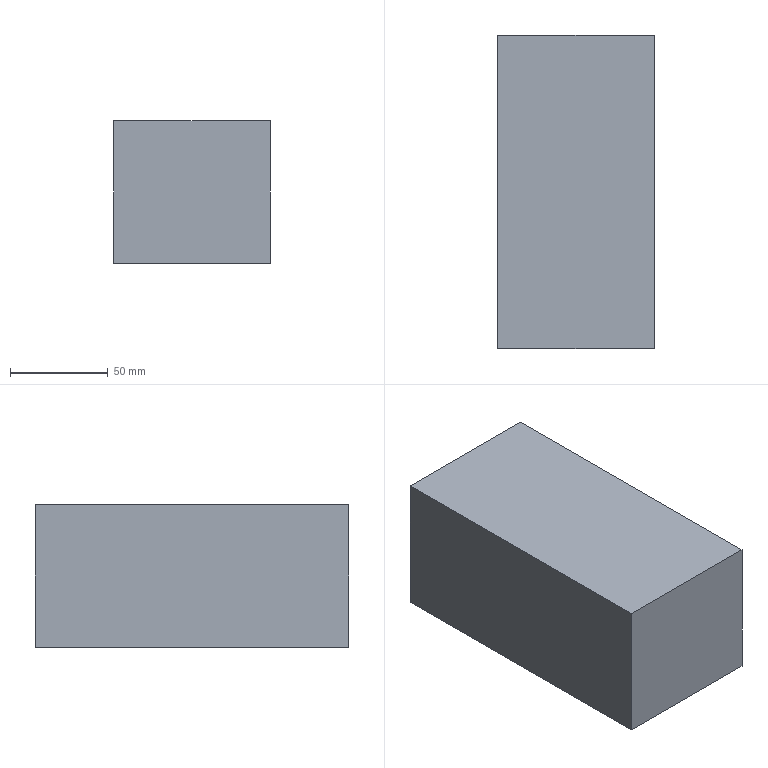Part | STEP file | 1 solid | 12 faces | box 80 x 160 x 72.8 mm | volume 929967 mm3 | plane 6 | cone 4 | cylinder 2 | commonest cylinder face diameters 6.8 x2
STEP:
#1=CARTESIAN_POINT('',(0.,0.,0.));
#2=DIRECTION('',(0.,0.,1.));
#3=DIRECTION('',(1.,0.,0.));
#4=AXIS2_PLACEMENT_3D('',#1,#2,#3);
#5=CARTESIAN_POINT('',(1936.247,362.48,-22.581));
#6=VERTEX_POINT('',#5);
#7=CARTESIAN_POINT('',(1856.247,362.48,-22.581));
#8=VERTEX_POINT('',#7);
#9=CARTESIAN_POINT('',(1956.247,362.48,-22.581));
#10=DIRECTION('',(-1.,0.,0.));
#11=VECTOR('',#10,1.);
#12=LINE('',#9,#11);
#13=CARTESIAN_POINT('',(1806.549,562.98,-22.581));
#14=DIRECTION('',(0.,0.,-1.));
#15=DIRECTION('',(-1.,0.,0.));
#16=AXIS2_PLACEMENT_3D('',#13,#14,#15);
#17=PLANE('',#16);
#18=CARTESIAN_POINT('',(-149.698,-200.5));
#19=DIRECTION('',(1.,0.));
#20=VECTOR('',#19,1.);
#21=LINE('',#18,#20);
#22=(GEOMETRIC_REPRESENTATION_CONTEXT(2)PARAMETRIC_REPRESENTATION_CONTEXT()REPRESENTATION_CONTEXT('',''));
#23=DEFINITIONAL_REPRESENTATION('',(#21),#22);
#24=PCURVE('',#17,#23);
#25=CARTESIAN_POINT('',(1956.247,362.48,-95.381));
#26=DIRECTION('',(0.,-1.,0.));
#27=DIRECTION('',(0.,0.,-1.));
#28=AXIS2_PLACEMENT_3D('',#25,#26,#27);
#29=PLANE('',#28);
#30=CARTESIAN_POINT('',(-72.8,0.));
#31=DIRECTION('',(0.,-1.));
#32=VECTOR('',#31,1.);
#33=LINE('',#30,#32);
#34=(GEOMETRIC_REPRESENTATION_CONTEXT(2)PARAMETRIC_REPRESENTATION_CONTEXT()REPRESENTATION_CONTEXT('',''));
#35=DEFINITIONAL_REPRESENTATION('',(#33),#34);
#36=PCURVE('',#29,#35);
#37=SURFACE_CURVE('',#12,(#24,#36),.PCURVE_S1.);
#38=EDGE_CURVE('',#6,#8,#37,.T.);
#39=ORIENTED_EDGE('',*,*,#38,.F.);
#40=CARTESIAN_POINT('',(1936.247,522.48,-22.581));
#41=VERTEX_POINT('',#40);
#42=CARTESIAN_POINT('',(1936.247,492.48,-22.581));
#43=DIRECTION('',(0.,-1.,0.));
#44=VECTOR('',#43,1.);
#45=LINE('',#42,#44);
#46=CARTESIAN_POINT('',(-129.698,-70.5));
#47=DIRECTION('',(0.,-1.));
#48=VECTOR('',#47,1.);
#49=LINE('',#46,#48);
#50=(GEOMETRIC_REPRESENTATION_CONTEXT(2)PARAMETRIC_REPRESENTATION_CONTEXT()REPRESENTATION_CONTEXT('',''));
#51=DEFINITIONAL_REPRESENTATION('',(#49),#50);
#52=PCURVE('',#17,#51);
#53=CARTESIAN_POINT('',(1936.247,492.48,-95.381));
#54=DIRECTION('',(1.,0.,0.));
#55=DIRECTION('',(0.,0.,1.));
#56=AXIS2_PLACEMENT_3D('',#53,#54,#55);
#57=PLANE('',#56);
#58=CARTESIAN_POINT('',(72.8,0.));
#59=DIRECTION('',(0.,1.));
#60=VECTOR('',#59,1.);
#61=LINE('',#58,#60);
#62=(GEOMETRIC_REPRESENTATION_CONTEXT(2)PARAMETRIC_REPRESENTATION_CONTEXT()REPRESENTATION_CONTEXT('',''));
#63=DEFINITIONAL_REPRESENTATION('',(#61),#62);
#64=PCURVE('',#57,#63);
#65=SURFACE_CURVE('',#45,(#52,#64),.PCURVE_S1.);
#66=EDGE_CURVE('',#41,#6,#65,.T.);
#67=ORIENTED_EDGE('',*,*,#66,.F.);
#68=CARTESIAN_POINT('',(1856.247,522.48,-22.581));
#69=VERTEX_POINT('',#68);
#70=CARTESIAN_POINT('',(1856.247,522.48,-22.581));
#71=DIRECTION('',(1.,0.,0.));
#72=VECTOR('',#71,1.);
#73=LINE('',#70,#72);
#74=CARTESIAN_POINT('',(-49.698,-40.5));
#75=DIRECTION('',(-1.,0.));
#76=VECTOR('',#75,1.);
#77=LINE('',#74,#76);
#78=(GEOMETRIC_REPRESENTATION_CONTEXT(2)PARAMETRIC_REPRESENTATION_CONTEXT()REPRESENTATION_CONTEXT('',''));
#79=DEFINITIONAL_REPRESENTATION('',(#77),#78);
#80=PCURVE('',#17,#79);
#81=CARTESIAN_POINT('',(1856.247,522.48,-95.381));
#82=DIRECTION('',(0.,1.,0.));
#83=DIRECTION('',(0.,0.,1.));
#84=AXIS2_PLACEMENT_3D('',#81,#82,#83);
#85=PLANE('',#84);
#86=CARTESIAN_POINT('',(72.8,0.));
#87=DIRECTION('',(0.,1.));
#88=VECTOR('',#87,1.);
#89=LINE('',#86,#88);
#90=(GEOMETRIC_REPRESENTATION_CONTEXT(2)PARAMETRIC_REPRESENTATION_CONTEXT()REPRESENTATION_CONTEXT('',''));
#91=DEFINITIONAL_REPRESENTATION('',(#89),#90);
#92=PCURVE('',#85,#91);
#93=SURFACE_CURVE('',#73,(#80,#92),.PCURVE_S1.);
#94=EDGE_CURVE('',#69,#41,#93,.T.);
#95=ORIENTED_EDGE('',*,*,#94,.F.);
#96=CARTESIAN_POINT('',(1856.247,392.48,-22.581));
#97=DIRECTION('',(0.,1.,0.));
#98=VECTOR('',#97,1.);
#99=LINE('',#96,#98);
#100=CARTESIAN_POINT('',(-49.698,-170.5));
#101=DIRECTION('',(0.,1.));
#102=VECTOR('',#101,1.);
#103=LINE('',#100,#102);
#104=(GEOMETRIC_REPRESENTATION_CONTEXT(2)PARAMETRIC_REPRESENTATION_CONTEXT()REPRESENTATION_CONTEXT('',''));
#105=DEFINITIONAL_REPRESENTATION('',(#103),#104);
#106=PCURVE('',#17,#105);
#107=CARTESIAN_POINT('',(1856.247,392.48,-95.381));
#108=DIRECTION('',(-1.,0.,0.));
#109=DIRECTION('',(0.,0.,-1.));
#110=AXIS2_PLACEMENT_3D('',#107,#108,#109);
#111=PLANE('',#110);
#112=CARTESIAN_POINT('',(-72.8,0.));
#113=DIRECTION('',(0.,-1.));
#114=VECTOR('',#113,1.);
#115=LINE('',#112,#114);
#116=(GEOMETRIC_REPRESENTATION_CONTEXT(2)PARAMETRIC_REPRESENTATION_CONTEXT()REPRESENTATION_CONTEXT('',''));
#117=DEFINITIONAL_REPRESENTATION('',(#115),#116);
#118=PCURVE('',#111,#117);
#119=SURFACE_CURVE('',#99,(#106,#118),.PCURVE_S1.);
#120=EDGE_CURVE('',#8,#69,#119,.T.);
#121=ORIENTED_EDGE('',*,*,#120,.F.);
#122=EDGE_LOOP('',(#39,#67,#95,#121));
#123=FACE_BOUND('',#122,.T.);
#124=ADVANCED_FACE('',(#123),#17,.F.);
#125=CARTESIAN_POINT('',(1856.247,522.48,-95.381));
#126=VERTEX_POINT('',#125);
#127=CARTESIAN_POINT('',(1856.247,522.48,-95.381));
#128=DIRECTION('',(0.,0.,-1.));
#129=VECTOR('',#128,1.);
#130=LINE('',#127,#129);
#131=CARTESIAN_POINT('',(0.,-130.));
#132=DIRECTION('',(1.,0.));
#133=VECTOR('',#132,1.);
#134=LINE('',#131,#133);
#135=(GEOMETRIC_REPRESENTATION_CONTEXT(2)PARAMETRIC_REPRESENTATION_CONTEXT()REPRESENTATION_CONTEXT('',''));
#136=DEFINITIONAL_REPRESENTATION('',(#134),#135);
#137=PCURVE('',#111,#136);
#138=CARTESIAN_POINT('',(0.,0.));
#139=DIRECTION('',(-1.,0.));
#140=VECTOR('',#139,1.);
#141=LINE('',#138,#140);
#142=(GEOMETRIC_REPRESENTATION_CONTEXT(2)PARAMETRIC_REPRESENTATION_CONTEXT()REPRESENTATION_CONTEXT('',''));
#143=DEFINITIONAL_REPRESENTATION('',(#141),#142);
#144=PCURVE('',#85,#143);
#145=SURFACE_CURVE('',#130,(#137,#144),.PCURVE_S1.);
#146=EDGE_CURVE('',#69,#126,#145,.T.);
#147=ORIENTED_EDGE('',*,*,#146,.T.);
#148=CARTESIAN_POINT('',(1856.247,362.48,-95.381));
#149=VERTEX_POINT('',#148);
#150=CARTESIAN_POINT('',(1856.247,392.48,-95.381));
#151=DIRECTION('',(0.,-1.,0.));
#152=VECTOR('',#151,1.);
#153=LINE('',#150,#152);
#154=CARTESIAN_POINT('',(0.,0.));
#155=DIRECTION('',(0.,1.));
#156=VECTOR('',#155,1.);
#157=LINE('',#154,#156);
#158=(GEOMETRIC_REPRESENTATION_CONTEXT(2)PARAMETRIC_REPRESENTATION_CONTEXT()REPRESENTATION_CONTEXT('',''));
#159=DEFINITIONAL_REPRESENTATION('',(#157),#158);
#160=PCURVE('',#111,#159);
#161=CARTESIAN_POINT('',(18457.433,-3577.789,-95.381));
#162=DIRECTION('',(0.,0.,1.));
#163=DIRECTION('',(-1.,0.,0.));
#164=AXIS2_PLACEMENT_3D('',#161,#162,#163);
#165=PLANE('',#164);
#166=CARTESIAN_POINT('',(16601.186,-3970.269));
#167=DIRECTION('',(0.,1.));
#168=VECTOR('',#167,1.);
#169=LINE('',#166,#168);
#170=(GEOMETRIC_REPRESENTATION_CONTEXT(2)PARAMETRIC_REPRESENTATION_CONTEXT()REPRESENTATION_CONTEXT('',''));
#171=DEFINITIONAL_REPRESENTATION('',(#169),#170);
#172=PCURVE('',#165,#171);
#173=SURFACE_CURVE('',#153,(#160,#172),.PCURVE_S1.);
#174=EDGE_CURVE('',#126,#149,#173,.T.);
#175=ORIENTED_EDGE('',*,*,#174,.T.);
#176=CARTESIAN_POINT('',(1856.247,362.48,-95.381));
#177=DIRECTION('',(0.,0.,-1.));
#178=VECTOR('',#177,1.);
#179=LINE('',#176,#178);
#180=CARTESIAN_POINT('',(0.,30.));
#181=DIRECTION('',(1.,0.));
#182=VECTOR('',#181,1.);
#183=LINE('',#180,#182);
#184=(GEOMETRIC_REPRESENTATION_CONTEXT(2)PARAMETRIC_REPRESENTATION_CONTEXT()REPRESENTATION_CONTEXT('',''));
#185=DEFINITIONAL_REPRESENTATION('',(#183),#184);
#186=PCURVE('',#111,#185);
#187=CARTESIAN_POINT('',(0.,-100.));
#188=DIRECTION('',(1.,0.));
#189=VECTOR('',#188,1.);
#190=LINE('',#187,#189);
#191=(GEOMETRIC_REPRESENTATION_CONTEXT(2)PARAMETRIC_REPRESENTATION_CONTEXT()REPRESENTATION_CONTEXT('',''));
#192=DEFINITIONAL_REPRESENTATION('',(#190),#191);
#193=PCURVE('',#29,#192);
#194=SURFACE_CURVE('',#179,(#186,#193),.PCURVE_S1.);
#195=EDGE_CURVE('',#8,#149,#194,.T.);
#196=ORIENTED_EDGE('',*,*,#195,.F.);
#197=ORIENTED_EDGE('',*,*,#120,.T.);
#198=EDGE_LOOP('',(#147,#175,#196,#197));
#199=FACE_BOUND('',#198,.T.);
#200=ADVANCED_FACE('',(#199),#111,.T.);
#201=CARTESIAN_POINT('',(1902.247,510.48,-95.381));
#202=VERTEX_POINT('',#201);
#203=CARTESIAN_POINT('',(1898.247,510.48,-95.381));
#204=DIRECTION('',(0.,0.,1.));
#205=DIRECTION('',(1.,0.,0.));
#206=AXIS2_PLACEMENT_3D('',#203,#204,#205);
#207=CIRCLE('',#206,4.);
#208=CARTESIAN_POINT('',(16559.186,-4088.269));
#209=DIRECTION('',(-1.,0.));
#210=AXIS2_PLACEMENT_2D('',#208,#209);
#211=CIRCLE('',#210,4.);
#212=(GEOMETRIC_REPRESENTATION_CONTEXT(2)PARAMETRIC_REPRESENTATION_CONTEXT()REPRESENTATION_CONTEXT('',''));
#213=DEFINITIONAL_REPRESENTATION('',(#211),#212);
#214=PCURVE('',#165,#213);
#215=CARTESIAN_POINT('',(1898.247,510.48,-95.381));
#216=DIRECTION('',(0.,0.,-1.));
#217=DIRECTION('',(-1.,0.,0.));
#218=AXIS2_PLACEMENT_3D('',#215,#216,#217);
#219=CONICAL_SURFACE('',#218,4.,0.7854);
#220=CARTESIAN_POINT('',(9.425,0.));
#221=DIRECTION('',(-1.,0.));
#222=VECTOR('',#221,1.);
#223=LINE('',#220,#222);
#224=(GEOMETRIC_REPRESENTATION_CONTEXT(2)PARAMETRIC_REPRESENTATION_CONTEXT()REPRESENTATION_CONTEXT('',''));
#225=DEFINITIONAL_REPRESENTATION('',(#223),#224);
#226=PCURVE('',#219,#225);
#227=SURFACE_CURVE('',#207,(#214,#226),.PCURVE_S1.);
#228=EDGE_CURVE('',#202,#202,#227,.T.);
#229=ORIENTED_EDGE('',*,*,#228,.T.);
#230=EDGE_LOOP('',(#229));
#231=FACE_BOUND('',#230,.T.);
#232=CARTESIAN_POINT('',(1902.247,374.48,-95.381));
#233=VERTEX_POINT('',#232);
#234=CARTESIAN_POINT('',(1898.247,374.48,-95.381));
#235=DIRECTION('',(0.,0.,1.));
#236=DIRECTION('',(1.,0.,0.));
#237=AXIS2_PLACEMENT_3D('',#234,#235,#236);
#238=CIRCLE('',#237,4.);
#239=CARTESIAN_POINT('',(16559.186,-3952.269));
#240=DIRECTION('',(-1.,0.));
#241=AXIS2_PLACEMENT_2D('',#239,#240);
#242=CIRCLE('',#241,4.);
#243=(GEOMETRIC_REPRESENTATION_CONTEXT(2)PARAMETRIC_REPRESENTATION_CONTEXT()REPRESENTATION_CONTEXT('',''));
#244=DEFINITIONAL_REPRESENTATION('',(#242),#243);
#245=PCURVE('',#165,#244);
#246=CARTESIAN_POINT('',(1898.247,374.48,-95.381));
#247=DIRECTION('',(0.,0.,-1.));
#248=DIRECTION('',(-1.,0.,0.));
#249=AXIS2_PLACEMENT_3D('',#246,#247,#248);
#250=CONICAL_SURFACE('',#249,4.,0.7854);
#251=CARTESIAN_POINT('',(9.425,0.));
#252=DIRECTION('',(-1.,0.));
#253=VECTOR('',#252,1.);
#254=LINE('',#251,#253);
#255=(GEOMETRIC_REPRESENTATION_CONTEXT(2)PARAMETRIC_REPRESENTATION_CONTEXT()REPRESENTATION_CONTEXT('',''));
#256=DEFINITIONAL_REPRESENTATION('',(#254),#255);
#257=PCURVE('',#250,#256);
#258=SURFACE_CURVE('',#238,(#245,#257),.PCURVE_S1.);
#259=EDGE_CURVE('',#233,#233,#258,.T.);
#260=ORIENTED_EDGE('',*,*,#259,.T.);
#261=EDGE_LOOP('',(#260));
#262=FACE_BOUND('',#261,.T.);
#263=CARTESIAN_POINT('',(1936.247,362.48,-95.381));
#264=VERTEX_POINT('',#263);
#265=CARTESIAN_POINT('',(18457.433,362.48,-95.381));
#266=DIRECTION('',(1.,0.,0.));
#267=VECTOR('',#266,1.);
#268=LINE('',#265,#267);
#269=CARTESIAN_POINT('',(0.,-3940.269));
#270=DIRECTION('',(-1.,0.));
#271=VECTOR('',#270,1.);
#272=LINE('',#269,#271);
#273=(GEOMETRIC_REPRESENTATION_CONTEXT(2)PARAMETRIC_REPRESENTATION_CONTEXT()REPRESENTATION_CONTEXT('',''));
#274=DEFINITIONAL_REPRESENTATION('',(#272),#273);
#275=PCURVE('',#165,#274);
#276=CARTESIAN_POINT('',(0.,16501.186));
#277=DIRECTION('',(0.,1.));
#278=VECTOR('',#277,1.);
#279=LINE('',#276,#278);
#280=(GEOMETRIC_REPRESENTATION_CONTEXT(2)PARAMETRIC_REPRESENTATION_CONTEXT()REPRESENTATION_CONTEXT('',''));
#281=DEFINITIONAL_REPRESENTATION('',(#279),#280);
#282=PCURVE('',#29,#281);
#283=SURFACE_CURVE('',#268,(#275,#282),.PCURVE_S1.);
#284=EDGE_CURVE('',#149,#264,#283,.T.);
#285=ORIENTED_EDGE('',*,*,#284,.F.);
#286=ORIENTED_EDGE('',*,*,#174,.F.);
#287=CARTESIAN_POINT('',(1936.247,522.48,-95.381));
#288=VERTEX_POINT('',#287);
#289=CARTESIAN_POINT('',(18457.433,522.48,-95.381));
#290=DIRECTION('',(-1.,0.,0.));
#291=VECTOR('',#290,1.);
#292=LINE('',#289,#291);
#293=CARTESIAN_POINT('',(0.,-4100.269));
#294=DIRECTION('',(1.,0.));
#295=VECTOR('',#294,1.);
#296=LINE('',#293,#295);
#297=(GEOMETRIC_REPRESENTATION_CONTEXT(2)PARAMETRIC_REPRESENTATION_CONTEXT()REPRESENTATION_CONTEXT('',''));
#298=DEFINITIONAL_REPRESENTATION('',(#296),#297);
#299=PCURVE('',#165,#298);
#300=CARTESIAN_POINT('',(0.,16601.186));
#301=DIRECTION('',(0.,-1.));
#302=VECTOR('',#301,1.);
#303=LINE('',#300,#302);
#304=(GEOMETRIC_REPRESENTATION_CONTEXT(2)PARAMETRIC_REPRESENTATION_CONTEXT()REPRESENTATION_CONTEXT('',''));
#305=DEFINITIONAL_REPRESENTATION('',(#303),#304);
#306=PCURVE('',#85,#305);
#307=SURFACE_CURVE('',#292,(#299,#306),.PCURVE_S1.);
#308=EDGE_CURVE('',#288,#126,#307,.T.);
#309=ORIENTED_EDGE('',*,*,#308,.F.);
#310=CARTESIAN_POINT('',(1936.247,-3577.789,-95.381));
#311=DIRECTION('',(0.,1.,0.));
#312=VECTOR('',#311,1.);
#313=LINE('',#310,#312);
#314=CARTESIAN_POINT('',(16521.186,0.));
#315=DIRECTION('',(0.,-1.));
#316=VECTOR('',#315,1.);
#317=LINE('',#314,#316);
#318=(GEOMETRIC_REPRESENTATION_CONTEXT(2)PARAMETRIC_REPRESENTATION_CONTEXT()REPRESENTATION_CONTEXT('',''));
#319=DEFINITIONAL_REPRESENTATION('',(#317),#318);
#320=PCURVE('',#165,#319);
#321=CARTESIAN_POINT('',(0.,4070.269));
#322=DIRECTION('',(0.,-1.));
#323=VECTOR('',#322,1.);
#324=LINE('',#321,#323);
#325=(GEOMETRIC_REPRESENTATION_CONTEXT(2)PARAMETRIC_REPRESENTATION_CONTEXT()REPRESENTATION_CONTEXT('',''));
#326=DEFINITIONAL_REPRESENTATION('',(#324),#325);
#327=PCURVE('',#57,#326);
#328=SURFACE_CURVE('',#313,(#320,#327),.PCURVE_S1.);
#329=EDGE_CURVE('',#264,#288,#328,.T.);
#330=ORIENTED_EDGE('',*,*,#329,.F.);
#331=EDGE_LOOP('',(#285,#286,#309,#330));
#332=FACE_BOUND('',#331,.T.);
#333=ADVANCED_FACE('',(#231,#262,#332),#165,.F.);
#334=CARTESIAN_POINT('',(1936.247,522.48,-95.381));
#335=DIRECTION('',(0.,0.,-1.));
#336=VECTOR('',#335,1.);
#337=LINE('',#334,#336);
#338=CARTESIAN_POINT('',(0.,80.));
#339=DIRECTION('',(-1.,0.));
#340=VECTOR('',#339,1.);
#341=LINE('',#338,#340);
#342=(GEOMETRIC_REPRESENTATION_CONTEXT(2)PARAMETRIC_REPRESENTATION_CONTEXT()REPRESENTATION_CONTEXT('',''));
#343=DEFINITIONAL_REPRESENTATION('',(#341),#342);
#344=PCURVE('',#85,#343);
#345=CARTESIAN_POINT('',(0.,-30.));
#346=DIRECTION('',(-1.,0.));
#347=VECTOR('',#346,1.);
#348=LINE('',#345,#347);
#349=(GEOMETRIC_REPRESENTATION_CONTEXT(2)PARAMETRIC_REPRESENTATION_CONTEXT()REPRESENTATION_CONTEXT('',''));
#350=DEFINITIONAL_REPRESENTATION('',(#348),#349);
#351=PCURVE('',#57,#350);
#352=SURFACE_CURVE('',#337,(#344,#351),.PCURVE_S1.);
#353=EDGE_CURVE('',#41,#288,#352,.T.);
#354=ORIENTED_EDGE('',*,*,#353,.T.);
#355=ORIENTED_EDGE('',*,*,#308,.T.);
#356=ORIENTED_EDGE('',*,*,#146,.F.);
#357=ORIENTED_EDGE('',*,*,#94,.T.);
#358=EDGE_LOOP('',(#354,#355,#356,#357));
#359=FACE_BOUND('',#358,.T.);
#360=ADVANCED_FACE('',(#359),#85,.T.);
#361=ORIENTED_EDGE('',*,*,#195,.T.);
#362=ORIENTED_EDGE('',*,*,#284,.T.);
#363=CARTESIAN_POINT('',(1936.247,362.48,-95.381));
#364=DIRECTION('',(0.,0.,-1.));
#365=VECTOR('',#364,1.);
#366=LINE('',#363,#365);
#367=CARTESIAN_POINT('',(0.,-20.));
#368=DIRECTION('',(1.,0.));
#369=VECTOR('',#368,1.);
#370=LINE('',#367,#369);
#371=(GEOMETRIC_REPRESENTATION_CONTEXT(2)PARAMETRIC_REPRESENTATION_CONTEXT()REPRESENTATION_CONTEXT('',''));
#372=DEFINITIONAL_REPRESENTATION('',(#370),#371);
#373=PCURVE('',#29,#372);
#374=CARTESIAN_POINT('',(0.,130.));
#375=DIRECTION('',(-1.,0.));
#376=VECTOR('',#375,1.);
#377=LINE('',#374,#376);
#378=(GEOMETRIC_REPRESENTATION_CONTEXT(2)PARAMETRIC_REPRESENTATION_CONTEXT()REPRESENTATION_CONTEXT('',''));
#379=DEFINITIONAL_REPRESENTATION('',(#377),#378);
#380=PCURVE('',#57,#379);
#381=SURFACE_CURVE('',#366,(#373,#380),.PCURVE_S1.);
#382=EDGE_CURVE('',#6,#264,#381,.T.);
#383=ORIENTED_EDGE('',*,*,#382,.F.);
#384=ORIENTED_EDGE('',*,*,#38,.T.);
#385=EDGE_LOOP('',(#361,#362,#383,#384));
#386=FACE_BOUND('',#385,.T.);
#387=ADVANCED_FACE('',(#386),#29,.T.);
#388=ORIENTED_EDGE('',*,*,#382,.T.);
#389=ORIENTED_EDGE('',*,*,#329,.T.);
#390=ORIENTED_EDGE('',*,*,#353,.F.);
#391=ORIENTED_EDGE('',*,*,#66,.T.);
#392=EDGE_LOOP('',(#388,#389,#390,#391));
#393=FACE_BOUND('',#392,.T.);
#394=ADVANCED_FACE('',(#393),#57,.T.);
#395=CARTESIAN_POINT('',(1894.847,374.48,-70.381));
#396=VERTEX_POINT('',#395);
#397=CARTESIAN_POINT('',(1901.647,374.48,-70.381));
#398=VERTEX_POINT('',#397);
#399=CARTESIAN_POINT('',(1898.247,374.48,-70.381));
#400=DIRECTION('',(0.,0.,-1.));
#401=DIRECTION('',(1.,0.,0.));
#402=AXIS2_PLACEMENT_3D('',#399,#400,#401);
#403=CIRCLE('',#402,3.4);
#404=CARTESIAN_POINT('',(1898.247,374.48,-70.381));
#405=DIRECTION('',(0.,0.,-1.));
#406=DIRECTION('',(-1.,0.,0.));
#407=AXIS2_PLACEMENT_3D('',#404,#405,#406);
#408=CONICAL_SURFACE('',#407,3.4,1.03);
#409=CARTESIAN_POINT('',(-3.142,0.));
#410=DIRECTION('',(1.,0.));
#411=VECTOR('',#410,1.);
#412=LINE('',#409,#411);
#413=(GEOMETRIC_REPRESENTATION_CONTEXT(2)PARAMETRIC_REPRESENTATION_CONTEXT()REPRESENTATION_CONTEXT('',''));
#414=DEFINITIONAL_REPRESENTATION('',(#412),#413);
#415=PCURVE('',#408,#414);
#416=CARTESIAN_POINT('',(1898.247,374.48,-95.381));
#417=DIRECTION('',(0.,0.,1.));
#418=DIRECTION('',(1.,0.,0.));
#419=AXIS2_PLACEMENT_3D('',#416,#417,#418);
#420=CYLINDRICAL_SURFACE('',#419,3.4);
#421=CARTESIAN_POINT('',(6.283,25.));
#422=DIRECTION('',(-1.,0.));
#423=VECTOR('',#422,1.);
#424=LINE('',#421,#423);
#425=(GEOMETRIC_REPRESENTATION_CONTEXT(2)PARAMETRIC_REPRESENTATION_CONTEXT()REPRESENTATION_CONTEXT('',''));
#426=DEFINITIONAL_REPRESENTATION('',(#424),#425);
#427=PCURVE('',#420,#426);
#428=SURFACE_CURVE('',#403,(#415,#427),.PCURVE_S1.);
#429=EDGE_CURVE('',#396,#398,#428,.T.);
#430=ORIENTED_EDGE('',*,*,#429,.F.);
#431=CARTESIAN_POINT('',(1898.247,374.48,-68.338));
#432=VERTEX_POINT('',#431);
#433=CARTESIAN_POINT('',(1898.247,374.48,-68.338));
#434=CARTESIAN_POINT('',(1894.847,374.48,-70.381));
#435=B_SPLINE_CURVE_WITH_KNOTS('',1,(#433,#434),.UNSPECIFIED.,.F.,.F.,(2,2),(-3.967,0.),.PIECEWISE_BEZIER_KNOTS.);
#436=CARTESIAN_POINT('',(0.,0.));
#437=DIRECTION('',(0.,1.));
#438=VECTOR('',#437,1.);
#439=LINE('',#436,#438);
#440=(GEOMETRIC_REPRESENTATION_CONTEXT(2)PARAMETRIC_REPRESENTATION_CONTEXT()REPRESENTATION_CONTEXT('',''));
#441=DEFINITIONAL_REPRESENTATION('',(#439),#440);
#442=PCURVE('',#408,#441);
#443=CARTESIAN_POINT('',(6.283,0.));
#444=DIRECTION('',(0.,1.));
#445=VECTOR('',#444,1.);
#446=LINE('',#443,#445);
#447=(GEOMETRIC_REPRESENTATION_CONTEXT(2)PARAMETRIC_REPRESENTATION_CONTEXT()REPRESENTATION_CONTEXT('',''));
#448=DEFINITIONAL_REPRESENTATION('',(#446),#447);
#449=PCURVE('',#408,#448);
#450=SEAM_CURVE('',#435,(#442,#449),.PCURVE_S1.);
#451=EDGE_CURVE('',#432,#396,#450,.T.);
#452=ORIENTED_EDGE('',*,*,#451,.F.);
#453=ORIENTED_EDGE('',*,*,#451,.T.);
#454=CARTESIAN_POINT('',(1898.247,374.48,-70.381));
#455=DIRECTION('',(0.,0.,-1.));
#456=DIRECTION('',(1.,0.,0.));
#457=AXIS2_PLACEMENT_3D('',#454,#455,#456);
#458=CIRCLE('',#457,3.4);
#459=CARTESIAN_POINT('',(3.142,0.));
#460=DIRECTION('',(1.,0.));
#461=VECTOR('',#460,1.);
#462=LINE('',#459,#461);
#463=(GEOMETRIC_REPRESENTATION_CONTEXT(2)PARAMETRIC_REPRESENTATION_CONTEXT()REPRESENTATION_CONTEXT('',''));
#464=DEFINITIONAL_REPRESENTATION('',(#462),#463);
#465=PCURVE('',#408,#464);
#466=CARTESIAN_POINT('',(6.283,25.));
#467=DIRECTION('',(-1.,0.));
#468=VECTOR('',#467,1.);
#469=LINE('',#466,#468);
#470=(GEOMETRIC_REPRESENTATION_CONTEXT(2)PARAMETRIC_REPRESENTATION_CONTEXT()REPRESENTATION_CONTEXT('',''));
#471=DEFINITIONAL_REPRESENTATION('',(#469),#470);
#472=PCURVE('',#420,#471);
#473=SURFACE_CURVE('',#458,(#465,#472),.PCURVE_S1.);
#474=EDGE_CURVE('',#398,#396,#473,.T.);
#475=ORIENTED_EDGE('',*,*,#474,.F.);
#476=EDGE_LOOP('',(#430,#452,#453,#475));
#477=FACE_BOUND('',#476,.F.);
#478=ADVANCED_FACE('',(#477),#408,.F.);
#479=CARTESIAN_POINT('',(1901.647,374.48,-94.781));
#480=VERTEX_POINT('',#479);
#481=CARTESIAN_POINT('',(1898.247,374.48,-94.781));
#482=DIRECTION('',(0.,0.,-1.));
#483=DIRECTION('',(1.,0.,0.));
#484=AXIS2_PLACEMENT_3D('',#481,#482,#483);
#485=CIRCLE('',#484,3.4);
#486=CARTESIAN_POINT('',(6.283,0.6));
#487=DIRECTION('',(-1.,0.));
#488=VECTOR('',#487,1.);
#489=LINE('',#486,#488);
#490=(GEOMETRIC_REPRESENTATION_CONTEXT(2)PARAMETRIC_REPRESENTATION_CONTEXT()REPRESENTATION_CONTEXT('',''));
#491=DEFINITIONAL_REPRESENTATION('',(#489),#490);
#492=PCURVE('',#420,#491);
#493=CARTESIAN_POINT('',(3.142,-0.6));
#494=DIRECTION('',(1.,0.));
#495=VECTOR('',#494,1.);
#496=LINE('',#493,#495);
#497=(GEOMETRIC_REPRESENTATION_CONTEXT(2)PARAMETRIC_REPRESENTATION_CONTEXT()REPRESENTATION_CONTEXT('',''));
#498=DEFINITIONAL_REPRESENTATION('',(#496),#497);
#499=PCURVE('',#250,#498);
#500=SURFACE_CURVE('',#485,(#492,#499),.PCURVE_S1.);
#501=EDGE_CURVE('',#480,#480,#500,.T.);
#502=ORIENTED_EDGE('',*,*,#501,.F.);
#503=CARTESIAN_POINT('',(1901.647,374.48,-94.781));
#504=CARTESIAN_POINT('',(1901.647,374.48,-70.381));
#505=B_SPLINE_CURVE_WITH_KNOTS('',1,(#503,#504),.UNSPECIFIED.,.F.,.F.,(2,2),(0.6,25.),.PIECEWISE_BEZIER_KNOTS.);
#506=CARTESIAN_POINT('',(6.283,0.));
#507=DIRECTION('',(0.,1.));
#508=VECTOR('',#507,1.);
#509=LINE('',#506,#508);
#510=(GEOMETRIC_REPRESENTATION_CONTEXT(2)PARAMETRIC_REPRESENTATION_CONTEXT()REPRESENTATION_CONTEXT('',''));
#511=DEFINITIONAL_REPRESENTATION('',(#509),#510);
#512=PCURVE('',#420,#511);
#513=CARTESIAN_POINT('',(0.,0.));
#514=DIRECTION('',(0.,1.));
#515=VECTOR('',#514,1.);
#516=LINE('',#513,#515);
#517=(GEOMETRIC_REPRESENTATION_CONTEXT(2)PARAMETRIC_REPRESENTATION_CONTEXT()REPRESENTATION_CONTEXT('',''));
#518=DEFINITIONAL_REPRESENTATION('',(#516),#517);
#519=PCURVE('',#420,#518);
#520=SEAM_CURVE('',#505,(#512,#519),.PCURVE_S1.);
#521=EDGE_CURVE('',#480,#398,#520,.T.);
#522=ORIENTED_EDGE('',*,*,#521,.T.);
#523=ORIENTED_EDGE('',*,*,#474,.T.);
#524=ORIENTED_EDGE('',*,*,#429,.T.);
#525=ORIENTED_EDGE('',*,*,#521,.F.);
#526=EDGE_LOOP('',(#502,#522,#523,#524,#525));
#527=FACE_BOUND('',#526,.F.);
#528=ADVANCED_FACE('',(#527),#420,.F.);
#529=ORIENTED_EDGE('',*,*,#501,.T.);
#530=CARTESIAN_POINT('',(1901.647,374.48,-94.781));
#531=CARTESIAN_POINT('',(1902.247,374.48,-95.381));
#532=B_SPLINE_CURVE_WITH_KNOTS('',1,(#530,#531),.UNSPECIFIED.,.F.,.F.,(2,2),(-0.8485,0.),.PIECEWISE_BEZIER_KNOTS.);
#533=CARTESIAN_POINT('',(9.425,0.));
#534=DIRECTION('',(0.,1.));
#535=VECTOR('',#534,1.);
#536=LINE('',#533,#535);
#537=(GEOMETRIC_REPRESENTATION_CONTEXT(2)PARAMETRIC_REPRESENTATION_CONTEXT()REPRESENTATION_CONTEXT('',''));
#538=DEFINITIONAL_REPRESENTATION('',(#536),#537);
#539=PCURVE('',#250,#538);
#540=CARTESIAN_POINT('',(3.142,0.));
#541=DIRECTION('',(0.,1.));
#542=VECTOR('',#541,1.);
#543=LINE('',#540,#542);
#544=(GEOMETRIC_REPRESENTATION_CONTEXT(2)PARAMETRIC_REPRESENTATION_CONTEXT()REPRESENTATION_CONTEXT('',''));
#545=DEFINITIONAL_REPRESENTATION('',(#543),#544);
#546=PCURVE('',#250,#545);
#547=SEAM_CURVE('',#532,(#539,#546),.PCURVE_S1.);
#548=EDGE_CURVE('',#480,#233,#547,.T.);
#549=ORIENTED_EDGE('',*,*,#548,.T.);
#550=ORIENTED_EDGE('',*,*,#259,.T.);
#551=ORIENTED_EDGE('',*,*,#548,.F.);
#552=EDGE_LOOP('',(#529,#549,#550,#551));
#553=FACE_BOUND('',#552,.F.);
#554=ADVANCED_FACE('',(#553),#250,.F.);
#555=CARTESIAN_POINT('',(1894.847,510.48,-70.381));
#556=VERTEX_POINT('',#555);
#557=CARTESIAN_POINT('',(1901.647,510.48,-70.381));
#558=VERTEX_POINT('',#557);
#559=CARTESIAN_POINT('',(1898.247,510.48,-70.381));
#560=DIRECTION('',(0.,0.,-1.));
#561=DIRECTION('',(1.,0.,0.));
#562=AXIS2_PLACEMENT_3D('',#559,#560,#561);
#563=CIRCLE('',#562,3.4);
#564=CARTESIAN_POINT('',(1898.247,510.48,-70.381));
#565=DIRECTION('',(0.,0.,-1.));
#566=DIRECTION('',(-1.,0.,0.));
#567=AXIS2_PLACEMENT_3D('',#564,#565,#566);
#568=CONICAL_SURFACE('',#567,3.4,1.03);
#569=CARTESIAN_POINT('',(-3.142,0.));
#570=DIRECTION('',(1.,0.));
#571=VECTOR('',#570,1.);
#572=LINE('',#569,#571);
#573=(GEOMETRIC_REPRESENTATION_CONTEXT(2)PARAMETRIC_REPRESENTATION_CONTEXT()REPRESENTATION_CONTEXT('',''));
#574=DEFINITIONAL_REPRESENTATION('',(#572),#573);
#575=PCURVE('',#568,#574);
#576=CARTESIAN_POINT('',(1898.247,510.48,-95.381));
#577=DIRECTION('',(0.,0.,1.));
#578=DIRECTION('',(1.,0.,0.));
#579=AXIS2_PLACEMENT_3D('',#576,#577,#578);
#580=CYLINDRICAL_SURFACE('',#579,3.4);
#581=CARTESIAN_POINT('',(6.283,25.));
#582=DIRECTION('',(-1.,0.));
#583=VECTOR('',#582,1.);
#584=LINE('',#581,#583);
#585=(GEOMETRIC_REPRESENTATION_CONTEXT(2)PARAMETRIC_REPRESENTATION_CONTEXT()REPRESENTATION_CONTEXT('',''));
#586=DEFINITIONAL_REPRESENTATION('',(#584),#585);
#587=PCURVE('',#580,#586);
#588=SURFACE_CURVE('',#563,(#575,#587),.PCURVE_S1.);
#589=EDGE_CURVE('',#556,#558,#588,.T.);
#590=ORIENTED_EDGE('',*,*,#589,.F.);
#591=CARTESIAN_POINT('',(1898.247,510.48,-68.338));
#592=VERTEX_POINT('',#591);
#593=CARTESIAN_POINT('',(1898.247,510.48,-68.338));
#594=CARTESIAN_POINT('',(1894.847,510.48,-70.381));
#595=B_SPLINE_CURVE_WITH_KNOTS('',1,(#593,#594),.UNSPECIFIED.,.F.,.F.,(2,2),(-3.967,0.),.PIECEWISE_BEZIER_KNOTS.);
#596=CARTESIAN_POINT('',(0.,0.));
#597=DIRECTION('',(0.,1.));
#598=VECTOR('',#597,1.);
#599=LINE('',#596,#598);
#600=(GEOMETRIC_REPRESENTATION_CONTEXT(2)PARAMETRIC_REPRESENTATION_CONTEXT()REPRESENTATION_CONTEXT('',''));
#601=DEFINITIONAL_REPRESENTATION('',(#599),#600);
#602=PCURVE('',#568,#601);
#603=CARTESIAN_POINT('',(6.283,0.));
#604=DIRECTION('',(0.,1.));
#605=VECTOR('',#604,1.);
#606=LINE('',#603,#605);
#607=(GEOMETRIC_REPRESENTATION_CONTEXT(2)PARAMETRIC_REPRESENTATION_CONTEXT()REPRESENTATION_CONTEXT('',''));
#608=DEFINITIONAL_REPRESENTATION('',(#606),#607);
#609=PCURVE('',#568,#608);
#610=SEAM_CURVE('',#595,(#602,#609),.PCURVE_S1.);
#611=EDGE_CURVE('',#592,#556,#610,.T.);
#612=ORIENTED_EDGE('',*,*,#611,.F.);
#613=ORIENTED_EDGE('',*,*,#611,.T.);
#614=CARTESIAN_POINT('',(1898.247,510.48,-70.381));
#615=DIRECTION('',(0.,0.,-1.));
#616=DIRECTION('',(1.,0.,0.));
#617=AXIS2_PLACEMENT_3D('',#614,#615,#616);
#618=CIRCLE('',#617,3.4);
#619=CARTESIAN_POINT('',(3.142,0.));
#620=DIRECTION('',(1.,0.));
#621=VECTOR('',#620,1.);
#622=LINE('',#619,#621);
#623=(GEOMETRIC_REPRESENTATION_CONTEXT(2)PARAMETRIC_REPRESENTATION_CONTEXT()REPRESENTATION_CONTEXT('',''));
#624=DEFINITIONAL_REPRESENTATION('',(#622),#623);
#625=PCURVE('',#568,#624);
#626=CARTESIAN_POINT('',(6.283,25.));
#627=DIRECTION('',(-1.,0.));
#628=VECTOR('',#627,1.);
#629=LINE('',#626,#628);
#630=(GEOMETRIC_REPRESENTATION_CONTEXT(2)PARAMETRIC_REPRESENTATION_CONTEXT()REPRESENTATION_CONTEXT('',''));
#631=DEFINITIONAL_REPRESENTATION('',(#629),#630);
#632=PCURVE('',#580,#631);
#633=SURFACE_CURVE('',#618,(#625,#632),.PCURVE_S1.);
#634=EDGE_CURVE('',#558,#556,#633,.T.);
#635=ORIENTED_EDGE('',*,*,#634,.F.);
#636=EDGE_LOOP('',(#590,#612,#613,#635));
#637=FACE_BOUND('',#636,.F.);
#638=ADVANCED_FACE('',(#637),#568,.F.);
#639=CARTESIAN_POINT('',(1901.647,510.48,-94.781));
#640=VERTEX_POINT('',#639);
#641=CARTESIAN_POINT('',(1898.247,510.48,-94.781));
#642=DIRECTION('',(0.,0.,-1.));
#643=DIRECTION('',(1.,0.,0.));
#644=AXIS2_PLACEMENT_3D('',#641,#642,#643);
#645=CIRCLE('',#644,3.4);
#646=CARTESIAN_POINT('',(6.283,0.6));
#647=DIRECTION('',(-1.,0.));
#648=VECTOR('',#647,1.);
#649=LINE('',#646,#648);
#650=(GEOMETRIC_REPRESENTATION_CONTEXT(2)PARAMETRIC_REPRESENTATION_CONTEXT()REPRESENTATION_CONTEXT('',''));
#651=DEFINITIONAL_REPRESENTATION('',(#649),#650);
#652=PCURVE('',#580,#651);
#653=CARTESIAN_POINT('',(3.142,-0.6));
#654=DIRECTION('',(1.,0.));
#655=VECTOR('',#654,1.);
#656=LINE('',#653,#655);
#657=(GEOMETRIC_REPRESENTATION_CONTEXT(2)PARAMETRIC_REPRESENTATION_CONTEXT()REPRESENTATION_CONTEXT('',''));
#658=DEFINITIONAL_REPRESENTATION('',(#656),#657);
#659=PCURVE('',#219,#658);
#660=SURFACE_CURVE('',#645,(#652,#659),.PCURVE_S1.);
#661=EDGE_CURVE('',#640,#640,#660,.T.);
#662=ORIENTED_EDGE('',*,*,#661,.F.);
#663=CARTESIAN_POINT('',(1901.647,510.48,-94.781));
#664=CARTESIAN_POINT('',(1901.647,510.48,-70.381));
#665=B_SPLINE_CURVE_WITH_KNOTS('',1,(#663,#664),.UNSPECIFIED.,.F.,.F.,(2,2),(0.6,25.),.PIECEWISE_BEZIER_KNOTS.);
#666=CARTESIAN_POINT('',(6.283,0.));
#667=DIRECTION('',(0.,1.));
#668=VECTOR('',#667,1.);
#669=LINE('',#666,#668);
#670=(GEOMETRIC_REPRESENTATION_CONTEXT(2)PARAMETRIC_REPRESENTATION_CONTEXT()REPRESENTATION_CONTEXT('',''));
#671=DEFINITIONAL_REPRESENTATION('',(#669),#670);
#672=PCURVE('',#580,#671);
#673=CARTESIAN_POINT('',(0.,0.));
#674=DIRECTION('',(0.,1.));
#675=VECTOR('',#674,1.);
#676=LINE('',#673,#675);
#677=(GEOMETRIC_REPRESENTATION_CONTEXT(2)PARAMETRIC_REPRESENTATION_CONTEXT()REPRESENTATION_CONTEXT('',''));
#678=DEFINITIONAL_REPRESENTATION('',(#676),#677);
#679=PCURVE('',#580,#678);
#680=SEAM_CURVE('',#665,(#672,#679),.PCURVE_S1.);
#681=EDGE_CURVE('',#640,#558,#680,.T.);
#682=ORIENTED_EDGE('',*,*,#681,.T.);
#683=ORIENTED_EDGE('',*,*,#634,.T.);
#684=ORIENTED_EDGE('',*,*,#589,.T.);
#685=ORIENTED_EDGE('',*,*,#681,.F.);
#686=EDGE_LOOP('',(#662,#682,#683,#684,#685));
#687=FACE_BOUND('',#686,.F.);
#688=ADVANCED_FACE('',(#687),#580,.F.);
#689=ORIENTED_EDGE('',*,*,#661,.T.);
#690=CARTESIAN_POINT('',(1901.647,510.48,-94.781));
#691=CARTESIAN_POINT('',(1902.247,510.48,-95.381));
#692=B_SPLINE_CURVE_WITH_KNOTS('',1,(#690,#691),.UNSPECIFIED.,.F.,.F.,(2,2),(-0.8485,0.),.PIECEWISE_BEZIER_KNOTS.);
#693=CARTESIAN_POINT('',(9.425,0.));
#694=DIRECTION('',(0.,1.));
#695=VECTOR('',#694,1.);
#696=LINE('',#693,#695);
#697=(GEOMETRIC_REPRESENTATION_CONTEXT(2)PARAMETRIC_REPRESENTATION_CONTEXT()REPRESENTATION_CONTEXT('',''));
#698=DEFINITIONAL_REPRESENTATION('',(#696),#697);
#699=PCURVE('',#219,#698);
#700=CARTESIAN_POINT('',(3.142,0.));
#701=DIRECTION('',(0.,1.));
#702=VECTOR('',#701,1.);
#703=LINE('',#700,#702);
#704=(GEOMETRIC_REPRESENTATION_CONTEXT(2)PARAMETRIC_REPRESENTATION_CONTEXT()REPRESENTATION_CONTEXT('',''));
#705=DEFINITIONAL_REPRESENTATION('',(#703),#704);
#706=PCURVE('',#219,#705);
#707=SEAM_CURVE('',#692,(#699,#706),.PCURVE_S1.);
#708=EDGE_CURVE('',#640,#202,#707,.T.);
#709=ORIENTED_EDGE('',*,*,#708,.T.);
#710=ORIENTED_EDGE('',*,*,#228,.T.);
#711=ORIENTED_EDGE('',*,*,#708,.F.);
#712=EDGE_LOOP('',(#689,#709,#710,#711));
#713=FACE_BOUND('',#712,.F.);
#714=ADVANCED_FACE('',(#713),#219,.F.);
#715=CLOSED_SHELL('',(#124,#200,#333,#360,#387,#394,#478,#528,#554,#638,#688,#714));
#716=MANIFOLD_SOLID_BREP('',#715);
#717=(LENGTH_UNIT()NAMED_UNIT(*)SI_UNIT(.MILLI.,.METRE.));
#718=UNCERTAINTY_MEASURE_WITH_UNIT(LENGTH_MEASURE(0.000005),#717,'','');
#719=(NAMED_UNIT(*)PLANE_ANGLE_UNIT()SI_UNIT($,.RADIAN.));
#720=(NAMED_UNIT(*)SI_UNIT($,.STERADIAN.)SOLID_ANGLE_UNIT());
#721=(GEOMETRIC_REPRESENTATION_CONTEXT(3)GLOBAL_UNCERTAINTY_ASSIGNED_CONTEXT((#718))GLOBAL_UNIT_ASSIGNED_CONTEXT((#717,#719,#720))REPRESENTATION_CONTEXT('',''));
#722=ADVANCED_BREP_SHAPE_REPRESENTATION('',(#4,#716),#721);